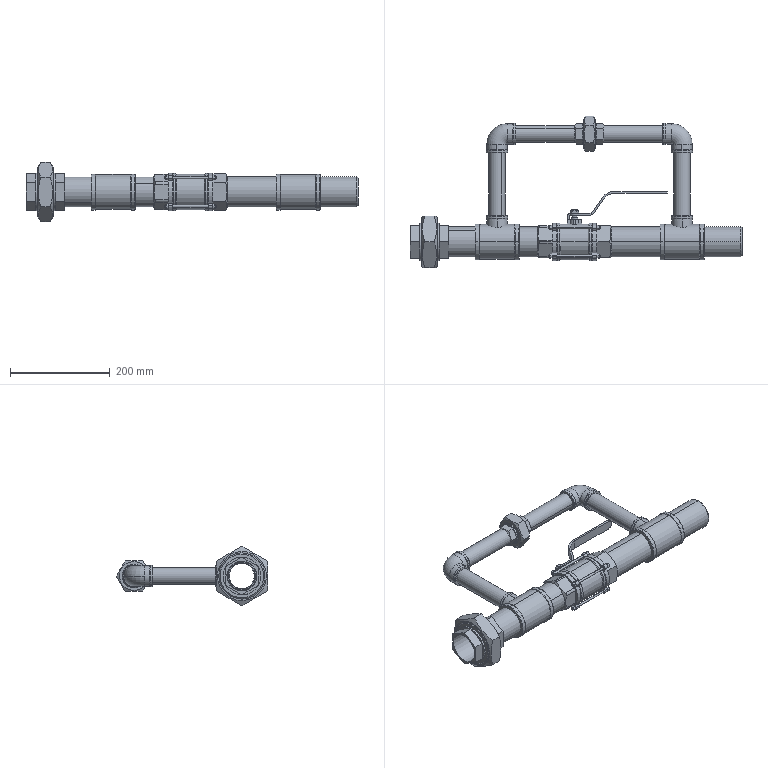Part | SolidWorks | 16 solids | 587 faces | box 664 x 302.792 x 119.17 mm | volume 1293430 mm3 | plane 245 | cylinder 196 | cone 94 | torus 52 | commonest cylinder face diameters 4.725 x24 33.5 x20 60 x18 75 x14 8.958 x12 41 x12